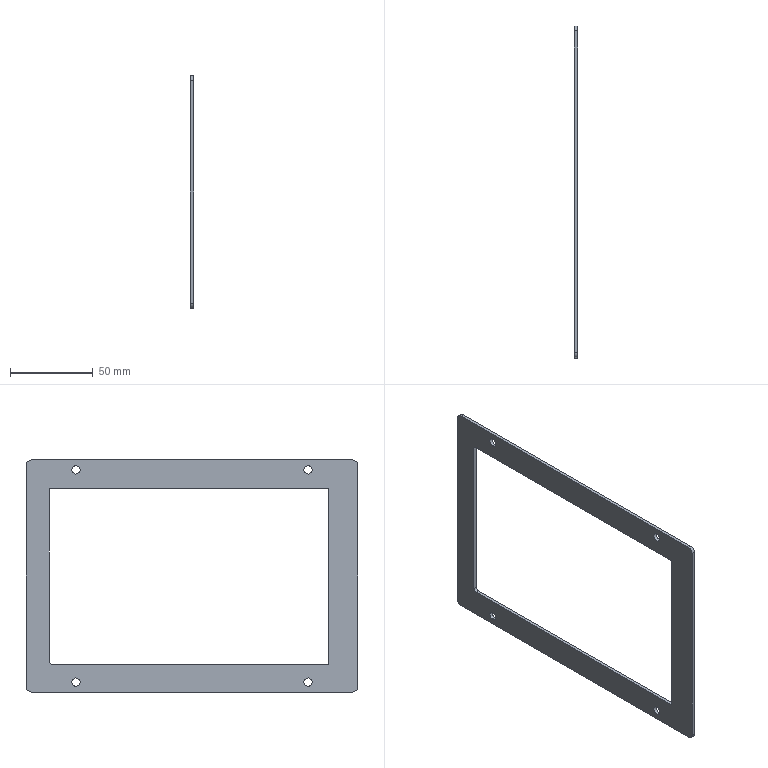Part | STEP file | RJ-HMS7-01_X2_58F34F5394A391D_2 | 1 solid | 24 faces | box 2 x 200 x 140 mm | volume 19939 mm3 | cylinder 14 | plane 10 | commonest cylinder face diameters 5 x8 6 x4 2 x1 4 x1